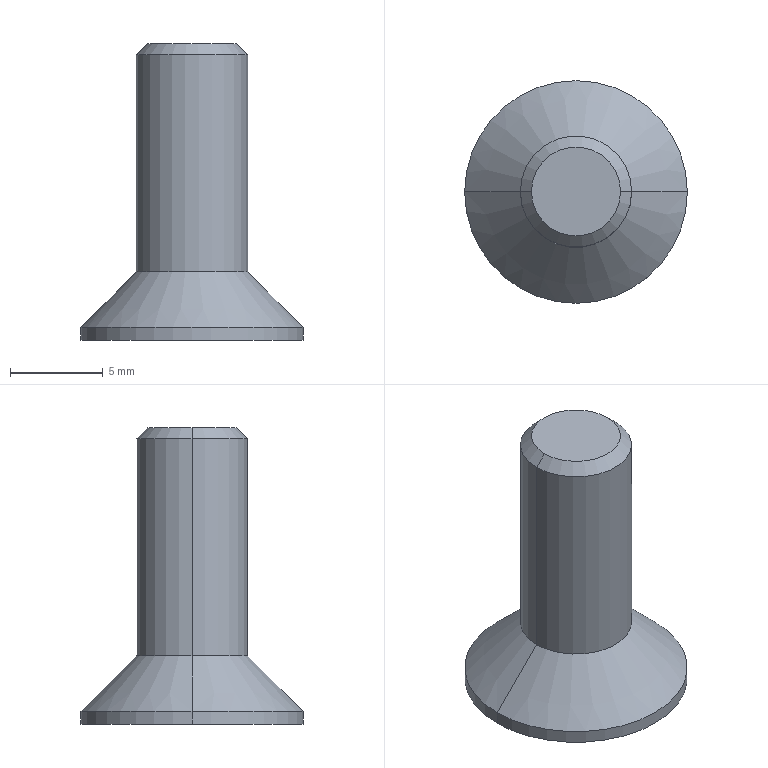Part | STEP file | LE-PJS-M6X16_PN_0003 | 1 solid | 24 faces | box 12 x 12 x 16 mm | volume 571.113 mm3 | plane 14 | cone 6 | cylinder 4 | commonest cylinder face diameters 6 x2 12 x2
STEP:
#1=CARTESIAN_POINT('',(-3.,0.,15.4));
#2=VERTEX_POINT('',#1);
#3=CARTESIAN_POINT('',(3.,0.,15.4));
#4=VERTEX_POINT('',#3);
#5=CARTESIAN_POINT('',(0.,0.,15.4));
#6=DIRECTION('',(0.,0.,-1.));
#7=DIRECTION('',(-1.,0.,0.));
#8=AXIS2_PLACEMENT_3D('',#5,#6,#7);
#9=CIRCLE('',#8,3.);
#10=EDGE_CURVE('',#2,#4,#9,.T.);
#11=ORIENTED_EDGE('',*,*,#10,.T.);
#12=CARTESIAN_POINT('',(3.,0.,3.7));
#13=VERTEX_POINT('',#12);
#14=CARTESIAN_POINT('',(3.,0.,16.));
#15=DIRECTION('',(0.,0.,-1.));
#16=VECTOR('',#15,1000.);
#17=LINE('',#14,#16);
#18=EDGE_CURVE('',#4,#13,#17,.T.);
#19=ORIENTED_EDGE('',*,*,#18,.T.);
#20=CARTESIAN_POINT('',(-3.,0.,3.7));
#21=VERTEX_POINT('',#20);
#22=CARTESIAN_POINT('',(0.,0.,3.7));
#23=DIRECTION('',(0.,0.,1.));
#24=DIRECTION('',(-1.,0.,0.));
#25=AXIS2_PLACEMENT_3D('',#22,#23,#24);
#26=CIRCLE('',#25,3.);
#27=EDGE_CURVE('',#13,#21,#26,.T.);
#28=ORIENTED_EDGE('',*,*,#27,.T.);
#29=CARTESIAN_POINT('',(-3.,0.,16.));
#30=DIRECTION('',(0.,0.,-1.));
#31=VECTOR('',#30,1000.);
#32=LINE('',#29,#31);
#33=EDGE_CURVE('',#2,#21,#32,.T.);
#34=ORIENTED_EDGE('',*,*,#33,.F.);
#35=EDGE_LOOP('',(#11,#19,#28,#34));
#36=FACE_OUTER_BOUND('',#35,.T.);
#37=CARTESIAN_POINT('',(0.,0.,16.));
#38=DIRECTION('',(0.,0.,-1.));
#39=DIRECTION('',(-1.,0.,0.));
#40=AXIS2_PLACEMENT_3D('',#37,#38,#39);
#41=CYLINDRICAL_SURFACE('',#40,3.);
#42=ADVANCED_FACE('',(#36),#41,.T.);
#43=ORIENTED_EDGE('',*,*,#27,.F.);
#44=CARTESIAN_POINT('',(6.,0.,0.7));
#45=VERTEX_POINT('',#44);
#46=CARTESIAN_POINT('',(6.,0.,0.7));
#47=DIRECTION('',(0.7071,0.,-0.7071));
#48=VECTOR('',#47,1000.);
#49=LINE('',#46,#48);
#50=EDGE_CURVE('',#13,#45,#49,.T.);
#51=ORIENTED_EDGE('',*,*,#50,.T.);
#52=CARTESIAN_POINT('',(-6.,0.,0.7));
#53=VERTEX_POINT('',#52);
#54=CARTESIAN_POINT('',(0.,0.,0.7));
#55=DIRECTION('',(0.,0.,1.));
#56=DIRECTION('',(-1.,0.,0.));
#57=AXIS2_PLACEMENT_3D('',#54,#55,#56);
#58=CIRCLE('',#57,6.);
#59=EDGE_CURVE('',#45,#53,#58,.T.);
#60=ORIENTED_EDGE('',*,*,#59,.T.);
#61=CARTESIAN_POINT('',(-6.,0.,0.7));
#62=DIRECTION('',(-0.7071,0.,-0.7071));
#63=VECTOR('',#62,1000.);
#64=LINE('',#61,#63);
#65=EDGE_CURVE('',#21,#53,#64,.T.);
#66=ORIENTED_EDGE('',*,*,#65,.F.);
#67=EDGE_LOOP('',(#43,#51,#60,#66));
#68=FACE_OUTER_BOUND('',#67,.T.);
#69=CARTESIAN_POINT('',(0.,0.,0.7));
#70=DIRECTION('',(0.,0.,-1.));
#71=DIRECTION('',(-1.,0.,0.));
#72=AXIS2_PLACEMENT_3D('',#69,#70,#71);
#73=CONICAL_SURFACE('',#72,6.,0.7854);
#74=ADVANCED_FACE('',(#68),#73,.T.);
#75=CARTESIAN_POINT('',(-2.4,0.,16.));
#76=VERTEX_POINT('',#75);
#77=CARTESIAN_POINT('',(2.4,0.,16.));
#78=VERTEX_POINT('',#77);
#79=CARTESIAN_POINT('',(0.,0.,16.));
#80=DIRECTION('',(0.,0.,-1.));
#81=DIRECTION('',(-1.,0.,0.));
#82=AXIS2_PLACEMENT_3D('',#79,#80,#81);
#83=CIRCLE('',#82,2.4);
#84=EDGE_CURVE('',#76,#78,#83,.T.);
#85=ORIENTED_EDGE('',*,*,#84,.T.);
#86=CARTESIAN_POINT('',(3.,0.,15.4));
#87=DIRECTION('',(0.7071,0.,-0.7071));
#88=VECTOR('',#87,1000.);
#89=LINE('',#86,#88);
#90=EDGE_CURVE('',#78,#4,#89,.T.);
#91=ORIENTED_EDGE('',*,*,#90,.T.);
#92=ORIENTED_EDGE('',*,*,#10,.F.);
#93=CARTESIAN_POINT('',(-3.,0.,15.4));
#94=DIRECTION('',(-0.7071,0.,-0.7071));
#95=VECTOR('',#94,1000.);
#96=LINE('',#93,#95);
#97=EDGE_CURVE('',#76,#2,#96,.T.);
#98=ORIENTED_EDGE('',*,*,#97,.F.);
#99=EDGE_LOOP('',(#85,#91,#92,#98));
#100=FACE_OUTER_BOUND('',#99,.T.);
#101=CARTESIAN_POINT('',(0.,0.,15.4));
#102=DIRECTION('',(0.,0.,-1.));
#103=DIRECTION('',(-1.,0.,0.));
#104=AXIS2_PLACEMENT_3D('',#101,#102,#103);
#105=CONICAL_SURFACE('',#104,3.,0.7854);
#106=ADVANCED_FACE('',(#100),#105,.T.);
#107=ORIENTED_EDGE('',*,*,#59,.F.);
#108=CARTESIAN_POINT('',(6.,0.,0.));
#109=VERTEX_POINT('',#108);
#110=CARTESIAN_POINT('',(6.,0.,3.7));
#111=DIRECTION('',(0.,0.,-1.));
#112=VECTOR('',#111,1000.);
#113=LINE('',#110,#112);
#114=EDGE_CURVE('',#45,#109,#113,.T.);
#115=ORIENTED_EDGE('',*,*,#114,.T.);
#116=CARTESIAN_POINT('',(-6.,0.,0.));
#117=VERTEX_POINT('',#116);
#118=CARTESIAN_POINT('',(0.,0.,0.));
#119=DIRECTION('',(0.,0.,1.));
#120=DIRECTION('',(-1.,0.,0.));
#121=AXIS2_PLACEMENT_3D('',#118,#119,#120);
#122=CIRCLE('',#121,6.);
#123=EDGE_CURVE('',#109,#117,#122,.T.);
#124=ORIENTED_EDGE('',*,*,#123,.T.);
#125=CARTESIAN_POINT('',(-6.,0.,3.7));
#126=DIRECTION('',(0.,0.,-1.));
#127=VECTOR('',#126,1000.);
#128=LINE('',#125,#127);
#129=EDGE_CURVE('',#53,#117,#128,.T.);
#130=ORIENTED_EDGE('',*,*,#129,.F.);
#131=EDGE_LOOP('',(#107,#115,#124,#130));
#132=FACE_OUTER_BOUND('',#131,.T.);
#133=CARTESIAN_POINT('',(0.,0.,3.7));
#134=DIRECTION('',(0.,0.,-1.));
#135=DIRECTION('',(-1.,0.,0.));
#136=AXIS2_PLACEMENT_3D('',#133,#134,#135);
#137=CYLINDRICAL_SURFACE('',#136,6.);
#138=ADVANCED_FACE('',(#132),#137,.T.);
#139=CARTESIAN_POINT('',(0.,0.,3.343));
#140=VERTEX_POINT('',#139);
#141=CARTESIAN_POINT('',(-2.5,0.,1.9));
#142=VERTEX_POINT('',#141);
#143=CARTESIAN_POINT('',(-2.5,0.,1.9));
#144=DIRECTION('',(-0.866,0.,-0.5));
#145=VECTOR('',#144,1000.);
#146=LINE('',#143,#145);
#147=EDGE_CURVE('',#140,#142,#146,.T.);
#148=ORIENTED_EDGE('',*,*,#147,.F.);
#149=CARTESIAN_POINT('',(2.5,0.,1.9));
#150=VERTEX_POINT('',#149);
#151=CARTESIAN_POINT('',(2.5,0.,1.9));
#152=DIRECTION('',(0.866,0.,-0.5));
#153=VECTOR('',#152,1000.);
#154=LINE('',#151,#153);
#155=EDGE_CURVE('',#140,#150,#154,.T.);
#156=ORIENTED_EDGE('',*,*,#155,.T.);
#157=CARTESIAN_POINT('',(2.165,-1.25,1.9));
#158=VERTEX_POINT('',#157);
#159=CARTESIAN_POINT('',(0.,0.,1.9));
#160=DIRECTION('',(0.,0.,1.));
#161=DIRECTION('',(-1.,0.,0.));
#162=AXIS2_PLACEMENT_3D('',#159,#160,#161);
#163=CIRCLE('',#162,2.5);
#164=EDGE_CURVE('',#158,#150,#163,.T.);
#165=ORIENTED_EDGE('',*,*,#164,.F.);
#166=CARTESIAN_POINT('',(0.,-2.5,1.9));
#167=VERTEX_POINT('',#166);
#168=CARTESIAN_POINT('',(0.,0.,1.9));
#169=DIRECTION('',(0.,0.,1.));
#170=DIRECTION('',(-1.,0.,0.));
#171=AXIS2_PLACEMENT_3D('',#168,#169,#170);
#172=CIRCLE('',#171,2.5);
#173=EDGE_CURVE('',#167,#158,#172,.T.);
#174=ORIENTED_EDGE('',*,*,#173,.F.);
#175=CARTESIAN_POINT('',(-2.165,-1.25,1.9));
#176=VERTEX_POINT('',#175);
#177=CARTESIAN_POINT('',(0.,0.,1.9));
#178=DIRECTION('',(0.,0.,1.));
#179=DIRECTION('',(-1.,0.,0.));
#180=AXIS2_PLACEMENT_3D('',#177,#178,#179);
#181=CIRCLE('',#180,2.5);
#182=EDGE_CURVE('',#176,#167,#181,.T.);
#183=ORIENTED_EDGE('',*,*,#182,.F.);
#184=CARTESIAN_POINT('',(0.,0.,1.9));
#185=DIRECTION('',(0.,0.,1.));
#186=DIRECTION('',(-1.,0.,0.));
#187=AXIS2_PLACEMENT_3D('',#184,#185,#186);
#188=CIRCLE('',#187,2.5);
#189=EDGE_CURVE('',#142,#176,#188,.T.);
#190=ORIENTED_EDGE('',*,*,#189,.F.);
#191=EDGE_LOOP('',(#148,#156,#165,#174,#183,#190));
#192=FACE_OUTER_BOUND('',#191,.T.);
#193=CARTESIAN_POINT('',(0.,0.,1.9));
#194=DIRECTION('',(0.,0.,-1.));
#195=DIRECTION('',(-1.,0.,0.));
#196=AXIS2_PLACEMENT_3D('',#193,#194,#195);
#197=CONICAL_SURFACE('',#196,2.5,1.047);
#198=ADVANCED_FACE('',(#192),#197,.F.);
#199=ORIENTED_EDGE('',*,*,#18,.F.);
#200=CARTESIAN_POINT('',(0.,0.,15.4));
#201=DIRECTION('',(0.,0.,-1.));
#202=DIRECTION('',(-1.,0.,0.));
#203=AXIS2_PLACEMENT_3D('',#200,#201,#202);
#204=CIRCLE('',#203,3.);
#205=EDGE_CURVE('',#4,#2,#204,.T.);
#206=ORIENTED_EDGE('',*,*,#205,.T.);
#207=ORIENTED_EDGE('',*,*,#33,.T.);
#208=CARTESIAN_POINT('',(0.,0.,3.7));
#209=DIRECTION('',(0.,0.,1.));
#210=DIRECTION('',(-1.,0.,0.));
#211=AXIS2_PLACEMENT_3D('',#208,#209,#210);
#212=CIRCLE('',#211,3.);
#213=EDGE_CURVE('',#21,#13,#212,.T.);
#214=ORIENTED_EDGE('',*,*,#213,.T.);
#215=EDGE_LOOP('',(#199,#206,#207,#214));
#216=FACE_OUTER_BOUND('',#215,.T.);
#217=CARTESIAN_POINT('',(0.,0.,16.));
#218=DIRECTION('',(0.,0.,-1.));
#219=DIRECTION('',(-1.,0.,0.));
#220=AXIS2_PLACEMENT_3D('',#217,#218,#219);
#221=CYLINDRICAL_SURFACE('',#220,3.);
#222=ADVANCED_FACE('',(#216),#221,.T.);
#223=ORIENTED_EDGE('',*,*,#50,.F.);
#224=ORIENTED_EDGE('',*,*,#213,.F.);
#225=ORIENTED_EDGE('',*,*,#65,.T.);
#226=CARTESIAN_POINT('',(0.,0.,0.7));
#227=DIRECTION('',(0.,0.,1.));
#228=DIRECTION('',(-1.,0.,0.));
#229=AXIS2_PLACEMENT_3D('',#226,#227,#228);
#230=CIRCLE('',#229,6.);
#231=EDGE_CURVE('',#53,#45,#230,.T.);
#232=ORIENTED_EDGE('',*,*,#231,.T.);
#233=EDGE_LOOP('',(#223,#224,#225,#232));
#234=FACE_OUTER_BOUND('',#233,.T.);
#235=CARTESIAN_POINT('',(0.,0.,0.7));
#236=DIRECTION('',(0.,0.,-1.));
#237=DIRECTION('',(-1.,0.,0.));
#238=AXIS2_PLACEMENT_3D('',#235,#236,#237);
#239=CONICAL_SURFACE('',#238,6.,0.7854);
#240=ADVANCED_FACE('',(#234),#239,.T.);
#241=ORIENTED_EDGE('',*,*,#90,.F.);
#242=CARTESIAN_POINT('',(0.,0.,16.));
#243=DIRECTION('',(0.,0.,-1.));
#244=DIRECTION('',(-1.,0.,0.));
#245=AXIS2_PLACEMENT_3D('',#242,#243,#244);
#246=CIRCLE('',#245,2.4);
#247=EDGE_CURVE('',#78,#76,#246,.T.);
#248=ORIENTED_EDGE('',*,*,#247,.T.);
#249=ORIENTED_EDGE('',*,*,#97,.T.);
#250=ORIENTED_EDGE('',*,*,#205,.F.);
#251=EDGE_LOOP('',(#241,#248,#249,#250));
#252=FACE_OUTER_BOUND('',#251,.T.);
#253=CARTESIAN_POINT('',(0.,0.,15.4));
#254=DIRECTION('',(0.,0.,-1.));
#255=DIRECTION('',(-1.,0.,0.));
#256=AXIS2_PLACEMENT_3D('',#253,#254,#255);
#257=CONICAL_SURFACE('',#256,3.,0.7854);
#258=ADVANCED_FACE('',(#252),#257,.T.);
#259=ORIENTED_EDGE('',*,*,#114,.F.);
#260=ORIENTED_EDGE('',*,*,#231,.F.);
#261=ORIENTED_EDGE('',*,*,#129,.T.);
#262=CARTESIAN_POINT('',(0.,0.,0.));
#263=DIRECTION('',(0.,0.,1.));
#264=DIRECTION('',(-1.,0.,0.));
#265=AXIS2_PLACEMENT_3D('',#262,#263,#264);
#266=CIRCLE('',#265,6.);
#267=EDGE_CURVE('',#117,#109,#266,.T.);
#268=ORIENTED_EDGE('',*,*,#267,.T.);
#269=EDGE_LOOP('',(#259,#260,#261,#268));
#270=FACE_OUTER_BOUND('',#269,.T.);
#271=CARTESIAN_POINT('',(0.,0.,3.7));
#272=DIRECTION('',(0.,0.,-1.));
#273=DIRECTION('',(-1.,0.,0.));
#274=AXIS2_PLACEMENT_3D('',#271,#272,#273);
#275=CYLINDRICAL_SURFACE('',#274,6.);
#276=ADVANCED_FACE('',(#270),#275,.T.);
#277=ORIENTED_EDGE('',*,*,#84,.F.);
#278=ORIENTED_EDGE('',*,*,#247,.F.);
#279=EDGE_LOOP('',(#277,#278));
#280=FACE_OUTER_BOUND('',#279,.T.);
#281=CARTESIAN_POINT('',(0.,0.,16.));
#282=DIRECTION('',(0.,0.,1.));
#283=DIRECTION('',(1.,0.,0.));
#284=AXIS2_PLACEMENT_3D('',#281,#282,#283);
#285=PLANE('',#284);
#286=ADVANCED_FACE('',(#280),#285,.T.);
#287=ORIENTED_EDGE('',*,*,#267,.F.);
#288=ORIENTED_EDGE('',*,*,#123,.F.);
#289=EDGE_LOOP('',(#287,#288));
#290=FACE_OUTER_BOUND('',#289,.T.);
#291=CARTESIAN_POINT('',(-2.887,0.,0.));
#292=VERTEX_POINT('',#291);
#293=CARTESIAN_POINT('',(-1.443,2.5,0.));
#294=VERTEX_POINT('',#293);
#295=CARTESIAN_POINT('',(-2.887,0.,0.));
#296=DIRECTION('',(0.5,0.866,0.));
#297=VECTOR('',#296,1000.);
#298=LINE('',#295,#297);
#299=EDGE_CURVE('',#292,#294,#298,.T.);
#300=ORIENTED_EDGE('',*,*,#299,.F.);
#301=CARTESIAN_POINT('',(-1.443,-2.5,0.));
#302=VERTEX_POINT('',#301);
#303=CARTESIAN_POINT('',(-1.443,-2.5,0.));
#304=DIRECTION('',(-0.5,0.866,0.));
#305=VECTOR('',#304,1000.);
#306=LINE('',#303,#305);
#307=EDGE_CURVE('',#302,#292,#306,.T.);
#308=ORIENTED_EDGE('',*,*,#307,.F.);
#309=CARTESIAN_POINT('',(1.443,-2.5,0.));
#310=VERTEX_POINT('',#309);
#311=CARTESIAN_POINT('',(0.,-2.5,0.));
#312=DIRECTION('',(-1.,0.,0.));
#313=VECTOR('',#312,1000.);
#314=LINE('',#311,#313);
#315=EDGE_CURVE('',#310,#302,#314,.T.);
#316=ORIENTED_EDGE('',*,*,#315,.F.);
#317=CARTESIAN_POINT('',(2.887,0.,0.));
#318=VERTEX_POINT('',#317);
#319=CARTESIAN_POINT('',(2.887,0.,0.));
#320=DIRECTION('',(-0.5,-0.866,0.));
#321=VECTOR('',#320,1000.);
#322=LINE('',#319,#321);
#323=EDGE_CURVE('',#318,#310,#322,.T.);
#324=ORIENTED_EDGE('',*,*,#323,.F.);
#325=CARTESIAN_POINT('',(1.443,2.5,0.));
#326=VERTEX_POINT('',#325);
#327=CARTESIAN_POINT('',(1.443,2.5,0.));
#328=DIRECTION('',(0.5,-0.866,0.));
#329=VECTOR('',#328,1000.);
#330=LINE('',#327,#329);
#331=EDGE_CURVE('',#326,#318,#330,.T.);
#332=ORIENTED_EDGE('',*,*,#331,.F.);
#333=CARTESIAN_POINT('',(0.,2.5,0.));
#334=DIRECTION('',(1.,0.,0.));
#335=VECTOR('',#334,1000.);
#336=LINE('',#333,#335);
#337=EDGE_CURVE('',#294,#326,#336,.T.);
#338=ORIENTED_EDGE('',*,*,#337,.F.);
#339=EDGE_LOOP('',(#300,#308,#316,#324,#332,#338));
#340=FACE_BOUND('',#339,.T.);
#341=CARTESIAN_POINT('',(0.,0.,0.));
#342=DIRECTION('',(0.,0.,1.));
#343=DIRECTION('',(1.,0.,0.));
#344=AXIS2_PLACEMENT_3D('',#341,#342,#343);
#345=PLANE('',#344);
#346=ADVANCED_FACE('',(#290,#340),#345,.F.);
#347=CARTESIAN_POINT('',(1.443,2.5,1.9));
#348=VERTEX_POINT('',#347);
#349=CARTESIAN_POINT('',(1.443,2.5,1.9));
#350=DIRECTION('',(0.,0.,-1.));
#351=VECTOR('',#350,1000.);
#352=LINE('',#349,#351);
#353=EDGE_CURVE('',#348,#326,#352,.T.);
#354=ORIENTED_EDGE('',*,*,#353,.F.);
#355=CARTESIAN_POINT('',(0.,2.5,1.9));
#356=VERTEX_POINT('',#355);
#357=CARTESIAN_POINT('',(0.,2.5,1.9));
#358=DIRECTION('',(1.,0.,0.));
#359=VECTOR('',#358,1000.);
#360=LINE('',#357,#359);
#361=EDGE_CURVE('',#356,#348,#360,.T.);
#362=ORIENTED_EDGE('',*,*,#361,.F.);
#363=CARTESIAN_POINT('',(-1.443,2.5,1.9));
#364=VERTEX_POINT('',#363);
#365=CARTESIAN_POINT('',(0.,2.5,1.9));
#366=DIRECTION('',(1.,0.,0.));
#367=VECTOR('',#366,1000.);
#368=LINE('',#365,#367);
#369=EDGE_CURVE('',#364,#356,#368,.T.);
#370=ORIENTED_EDGE('',*,*,#369,.F.);
#371=CARTESIAN_POINT('',(-1.443,2.5,1.9));
#372=DIRECTION('',(0.,0.,1.));
#373=VECTOR('',#372,1000.);
#374=LINE('',#371,#373);
#375=EDGE_CURVE('',#294,#364,#374,.T.);
#376=ORIENTED_EDGE('',*,*,#375,.F.);
#377=ORIENTED_EDGE('',*,*,#337,.T.);
#378=EDGE_LOOP('',(#354,#362,#370,#376,#377));
#379=FACE_OUTER_BOUND('',#378,.T.);
#380=CARTESIAN_POINT('',(-1.443,2.5,1.9));
#381=DIRECTION('',(0.,1.,0.));
#382=DIRECTION('',(0.,0.,1.));
#383=AXIS2_PLACEMENT_3D('',#380,#381,#382);
#384=PLANE('',#383);
#385=ADVANCED_FACE('',(#379),#384,.F.);
#386=ORIENTED_EDGE('',*,*,#375,.T.);
#387=CARTESIAN_POINT('',(-2.165,1.25,1.9));
#388=VERTEX_POINT('',#387);
#389=CARTESIAN_POINT('',(-2.165,1.25,1.9));
#390=DIRECTION('',(0.5,0.866,0.));
#391=VECTOR('',#390,1000.);
#392=LINE('',#389,#391);
#393=EDGE_CURVE('',#388,#364,#392,.T.);
#394=ORIENTED_EDGE('',*,*,#393,.F.);
#395=CARTESIAN_POINT('',(-2.887,0.,1.9));
#396=VERTEX_POINT('',#395);
#397=CARTESIAN_POINT('',(-2.887,0.,1.9));
#398=DIRECTION('',(0.5,0.866,0.));
#399=VECTOR('',#398,1000.);
#400=LINE('',#397,#399);
#401=EDGE_CURVE('',#396,#388,#400,.T.);
#402=ORIENTED_EDGE('',*,*,#401,.F.);
#403=CARTESIAN_POINT('',(-2.887,0.,1.9));
#404=DIRECTION('',(0.,0.,1.));
#405=VECTOR('',#404,1000.);
#406=LINE('',#403,#405);
#407=EDGE_CURVE('',#292,#396,#406,.T.);
#408=ORIENTED_EDGE('',*,*,#407,.F.);
#409=ORIENTED_EDGE('',*,*,#299,.T.);
#410=EDGE_LOOP('',(#386,#394,#402,#408,#409));
#411=FACE_OUTER_BOUND('',#410,.T.);
#412=CARTESIAN_POINT('',(-2.887,0.,1.9));
#413=DIRECTION('',(-0.866,0.5,0.));
#414=DIRECTION('',(-0.5,-0.866,0.));
#415=AXIS2_PLACEMENT_3D('',#412,#413,#414);
#416=PLANE('',#415);
#417=ADVANCED_FACE('',(#411),#416,.F.);
#418=ORIENTED_EDGE('',*,*,#407,.T.);
#419=CARTESIAN_POINT('',(-1.443,-2.5,1.9));
#420=DIRECTION('',(-0.5,0.866,0.));
#421=VECTOR('',#420,1000.);
#422=LINE('',#419,#421);
#423=EDGE_CURVE('',#176,#396,#422,.T.);
#424=ORIENTED_EDGE('',*,*,#423,.F.);
#425=CARTESIAN_POINT('',(-1.443,-2.5,1.9));
#426=VERTEX_POINT('',#425);
#427=CARTESIAN_POINT('',(-1.443,-2.5,1.9));
#428=DIRECTION('',(-0.5,0.866,0.));
#429=VECTOR('',#428,1000.);
#430=LINE('',#427,#429);
#431=EDGE_CURVE('',#426,#176,#430,.T.);
#432=ORIENTED_EDGE('',*,*,#431,.F.);
#433=CARTESIAN_POINT('',(-1.443,-2.5,1.9));
#434=DIRECTION('',(0.,0.,1.));
#435=VECTOR('',#434,1000.);
#436=LINE('',#433,#435);
#437=EDGE_CURVE('',#302,#426,#436,.T.);
#438=ORIENTED_EDGE('',*,*,#437,.F.);
#439=ORIENTED_EDGE('',*,*,#307,.T.);
#440=EDGE_LOOP('',(#418,#424,#432,#438,#439));
#441=FACE_OUTER_BOUND('',#440,.T.);
#442=CARTESIAN_POINT('',(-1.443,-2.5,1.9));
#443=DIRECTION('',(-0.866,-0.5,0.));
#444=DIRECTION('',(0.5,-0.866,0.));
#445=AXIS2_PLACEMENT_3D('',#442,#443,#444);
#446=PLANE('',#445);
#447=ADVANCED_FACE('',(#441),#446,.F.);
#448=ORIENTED_EDGE('',*,*,#437,.T.);
#449=CARTESIAN_POINT('',(0.,-2.5,1.9));
#450=DIRECTION('',(-1.,0.,0.));
#451=VECTOR('',#450,1000.);
#452=LINE('',#449,#451);
#453=EDGE_CURVE('',#167,#426,#452,.T.);
#454=ORIENTED_EDGE('',*,*,#453,.F.);
#455=CARTESIAN_POINT('',(1.443,-2.5,1.9));
#456=VERTEX_POINT('',#455);
#457=CARTESIAN_POINT('',(0.,-2.5,1.9));
#458=DIRECTION('',(-1.,0.,0.));
#459=VECTOR('',#458,1000.);
#460=LINE('',#457,#459);
#461=EDGE_CURVE('',#456,#167,#460,.T.);
#462=ORIENTED_EDGE('',*,*,#461,.F.);
#463=CARTESIAN_POINT('',(1.443,-2.5,1.9));
#464=DIRECTION('',(0.,0.,1.));
#465=VECTOR('',#464,1000.);
#466=LINE('',#463,#465);
#467=EDGE_CURVE('',#310,#456,#466,.T.);
#468=ORIENTED_EDGE('',*,*,#467,.F.);
#469=ORIENTED_EDGE('',*,*,#315,.T.);
#470=EDGE_LOOP('',(#448,#454,#462,#468,#469));
#471=FACE_OUTER_BOUND('',#470,.T.);
#472=CARTESIAN_POINT('',(1.443,-2.5,1.9));
#473=DIRECTION('',(0.,-1.,0.));
#474=DIRECTION('',(1.,0.,0.));
#475=AXIS2_PLACEMENT_3D('',#472,#473,#474);
#476=PLANE('',#475);
#477=ADVANCED_FACE('',(#471),#476,.F.);
#478=ORIENTED_EDGE('',*,*,#467,.T.);
#479=CARTESIAN_POINT('',(2.165,-1.25,1.9));
#480=DIRECTION('',(-0.5,-0.866,0.));
#481=VECTOR('',#480,1000.);
#482=LINE('',#479,#481);
#483=EDGE_CURVE('',#158,#456,#482,.T.);
#484=ORIENTED_EDGE('',*,*,#483,.F.);
#485=CARTESIAN_POINT('',(2.887,0.,1.9));
#486=VERTEX_POINT('',#485);
#487=CARTESIAN_POINT('',(2.887,0.,1.9));
#488=DIRECTION('',(-0.5,-0.866,0.));
#489=VECTOR('',#488,1000.);
#490=LINE('',#487,#489);
#491=EDGE_CURVE('',#486,#158,#490,.T.);
#492=ORIENTED_EDGE('',*,*,#491,.F.);
#493=CARTESIAN_POINT('',(2.887,0.,1.9));
#494=DIRECTION('',(0.,0.,1.));
#495=VECTOR('',#494,1000.);
#496=LINE('',#493,#495);
#497=EDGE_CURVE('',#318,#486,#496,.T.);
#498=ORIENTED_EDGE('',*,*,#497,.F.);
#499=ORIENTED_EDGE('',*,*,#323,.T.);
#500=EDGE_LOOP('',(#478,#484,#492,#498,#499));
#501=FACE_OUTER_BOUND('',#500,.T.);
#502=CARTESIAN_POINT('',(2.887,0.,1.9));
#503=DIRECTION('',(0.866,-0.5,0.));
#504=DIRECTION('',(0.5,0.866,0.));
#505=AXIS2_PLACEMENT_3D('',#502,#503,#504);
#506=PLANE('',#505);
#507=ADVANCED_FACE('',(#501),#506,.F.);
#508=ORIENTED_EDGE('',*,*,#497,.T.);
#509=CARTESIAN_POINT('',(2.165,1.25,1.9));
#510=VERTEX_POINT('',#509);
#511=CARTESIAN_POINT('',(1.443,2.5,1.9));
#512=DIRECTION('',(0.5,-0.866,0.));
#513=VECTOR('',#512,1000.);
#514=LINE('',#511,#513);
#515=EDGE_CURVE('',#510,#486,#514,.T.);
#516=ORIENTED_EDGE('',*,*,#515,.F.);
#517=CARTESIAN_POINT('',(1.443,2.5,1.9));
#518=DIRECTION('',(0.5,-0.866,0.));
#519=VECTOR('',#518,1000.);
#520=LINE('',#517,#519);
#521=EDGE_CURVE('',#348,#510,#520,.T.);
#522=ORIENTED_EDGE('',*,*,#521,.F.);
#523=ORIENTED_EDGE('',*,*,#353,.T.);
#524=ORIENTED_EDGE('',*,*,#331,.T.);
#525=EDGE_LOOP('',(#508,#516,#522,#523,#524));
#526=FACE_OUTER_BOUND('',#525,.T.);
#527=CARTESIAN_POINT('',(1.443,2.5,1.9));
#528=DIRECTION('',(0.866,0.5,0.));
#529=DIRECTION('',(-0.5,0.866,0.));
#530=AXIS2_PLACEMENT_3D('',#527,#528,#529);
#531=PLANE('',#530);
#532=ADVANCED_FACE('',(#526),#531,.F.);
#533=ORIENTED_EDGE('',*,*,#401,.T.);
#534=CARTESIAN_POINT('',(0.,0.,1.9));
#535=DIRECTION('',(0.,0.,1.));
#536=DIRECTION('',(-1.,0.,0.));
#537=AXIS2_PLACEMENT_3D('',#534,#535,#536);
#538=CIRCLE('',#537,2.5);
#539=EDGE_CURVE('',#388,#142,#538,.T.);
#540=ORIENTED_EDGE('',*,*,#539,.T.);
#541=ORIENTED_EDGE('',*,*,#189,.T.);
#542=ORIENTED_EDGE('',*,*,#423,.T.);
#543=EDGE_LOOP('',(#533,#540,#541,#542));
#544=FACE_OUTER_BOUND('',#543,.T.);
#545=CARTESIAN_POINT('',(0.,0.,1.9));
#546=DIRECTION('',(0.,0.,-1.));
#547=DIRECTION('',(-1.,0.,0.));
#548=AXIS2_PLACEMENT_3D('',#545,#546,#547);
#549=PLANE('',#548);
#550=ADVANCED_FACE('',(#544),#549,.T.);
#551=ORIENTED_EDGE('',*,*,#491,.T.);
#552=ORIENTED_EDGE('',*,*,#164,.T.);
#553=CARTESIAN_POINT('',(0.,0.,1.9));
#554=DIRECTION('',(0.,0.,1.));
#555=DIRECTION('',(-1.,0.,0.));
#556=AXIS2_PLACEMENT_3D('',#553,#554,#555);
#557=CIRCLE('',#556,2.5);
#558=EDGE_CURVE('',#150,#510,#557,.T.);
#559=ORIENTED_EDGE('',*,*,#558,.T.);
#560=ORIENTED_EDGE('',*,*,#515,.T.);
#561=EDGE_LOOP('',(#551,#552,#559,#560));
#562=FACE_OUTER_BOUND('',#561,.T.);
#563=CARTESIAN_POINT('',(0.,0.,1.9));
#564=DIRECTION('',(0.,0.,-1.));
#565=DIRECTION('',(-1.,0.,0.));
#566=AXIS2_PLACEMENT_3D('',#563,#564,#565);
#567=PLANE('',#566);
#568=ADVANCED_FACE('',(#562),#567,.T.);
#569=ORIENTED_EDGE('',*,*,#361,.T.);
#570=ORIENTED_EDGE('',*,*,#521,.T.);
#571=CARTESIAN_POINT('',(0.,0.,1.9));
#572=DIRECTION('',(0.,0.,1.));
#573=DIRECTION('',(-1.,0.,0.));
#574=AXIS2_PLACEMENT_3D('',#571,#572,#573);
#575=CIRCLE('',#574,2.5);
#576=EDGE_CURVE('',#510,#356,#575,.T.);
#577=ORIENTED_EDGE('',*,*,#576,.T.);
#578=EDGE_LOOP('',(#569,#570,#577));
#579=FACE_OUTER_BOUND('',#578,.T.);
#580=CARTESIAN_POINT('',(0.,0.,1.9));
#581=DIRECTION('',(0.,0.,-1.));
#582=DIRECTION('',(-1.,0.,0.));
#583=AXIS2_PLACEMENT_3D('',#580,#581,#582);
#584=PLANE('',#583);
#585=ADVANCED_FACE('',(#579),#584,.T.);
#586=ORIENTED_EDGE('',*,*,#155,.F.);
#587=ORIENTED_EDGE('',*,*,#147,.T.);
#588=ORIENTED_EDGE('',*,*,#539,.F.);
#589=CARTESIAN_POINT('',(0.,0.,1.9));
#590=DIRECTION('',(0.,0.,1.));
#591=DIRECTION('',(-1.,0.,0.));
#592=AXIS2_PLACEMENT_3D('',#589,#590,#591);
#593=CIRCLE('',#592,2.5);
#594=EDGE_CURVE('',#356,#388,#593,.T.);
#595=ORIENTED_EDGE('',*,*,#594,.F.);
#596=ORIENTED_EDGE('',*,*,#576,.F.);
#597=ORIENTED_EDGE('',*,*,#558,.F.);
#598=EDGE_LOOP('',(#586,#587,#588,#595,#596,#597));
#599=FACE_OUTER_BOUND('',#598,.T.);
#600=CARTESIAN_POINT('',(0.,0.,1.9));
#601=DIRECTION('',(0.,0.,-1.));
#602=DIRECTION('',(-1.,0.,0.));
#603=AXIS2_PLACEMENT_3D('',#600,#601,#602);
#604=CONICAL_SURFACE('',#603,2.5,1.047);
#605=ADVANCED_FACE('',(#599),#604,.F.);
#606=ORIENTED_EDGE('',*,*,#393,.T.);
#607=ORIENTED_EDGE('',*,*,#369,.T.);
#608=ORIENTED_EDGE('',*,*,#594,.T.);
#609=EDGE_LOOP('',(#606,#607,#608));
#610=FACE_OUTER_BOUND('',#609,.T.);
#611=CARTESIAN_POINT('',(0.,0.,1.9));
#612=DIRECTION('',(0.,0.,-1.));
#613=DIRECTION('',(-1.,0.,0.));
#614=AXIS2_PLACEMENT_3D('',#611,#612,#613);
#615=PLANE('',#614);
#616=ADVANCED_FACE('',(#610),#615,.T.);
#617=ORIENTED_EDGE('',*,*,#483,.T.);
#618=ORIENTED_EDGE('',*,*,#461,.T.);
#619=ORIENTED_EDGE('',*,*,#173,.T.);
#620=EDGE_LOOP('',(#617,#618,#619));
#621=FACE_OUTER_BOUND('',#620,.T.);
#622=CARTESIAN_POINT('',(0.,0.,1.9));
#623=DIRECTION('',(0.,0.,-1.));
#624=DIRECTION('',(-1.,0.,0.));
#625=AXIS2_PLACEMENT_3D('',#622,#623,#624);
#626=PLANE('',#625);
#627=ADVANCED_FACE('',(#621),#626,.T.);
#628=ORIENTED_EDGE('',*,*,#453,.T.);
#629=ORIENTED_EDGE('',*,*,#431,.T.);
#630=ORIENTED_EDGE('',*,*,#182,.T.);
#631=EDGE_LOOP('',(#628,#629,#630));
#632=FACE_OUTER_BOUND('',#631,.T.);
#633=CARTESIAN_POINT('',(0.,0.,1.9));
#634=DIRECTION('',(0.,0.,-1.));
#635=DIRECTION('',(-1.,0.,0.));
#636=AXIS2_PLACEMENT_3D('',#633,#634,#635);
#637=PLANE('',#636);
#638=ADVANCED_FACE('',(#632),#637,.T.);
#639=CLOSED_SHELL('',(#42,#74,#106,#138,#198,#222,#240,#258,#276,#286,#346,#385,#417,#447,#477,#507,#532,#550,#568,#585,#605,#616,#627,#638));
#640=MANIFOLD_SOLID_BREP('',#639);
#641=CARTESIAN_POINT('',(0.,0.,0.));
#642=DIRECTION('',(0.,0.,1.));
#643=DIRECTION('',(1.,0.,0.));
#644=AXIS2_PLACEMENT_3D('',#641,#642,#643);
#645=(LENGTH_UNIT()NAMED_UNIT(*)SI_UNIT(.MILLI.,.METRE.));
#646=UNCERTAINTY_MEASURE_WITH_UNIT(LENGTH_MEASURE(0.00001),#645,'','');
#647=(NAMED_UNIT(*)PLANE_ANGLE_UNIT()SI_UNIT($,.RADIAN.));
#648=(NAMED_UNIT(*)SI_UNIT($,.STERADIAN.)SOLID_ANGLE_UNIT());
#649=(GEOMETRIC_REPRESENTATION_CONTEXT(3)GLOBAL_UNCERTAINTY_ASSIGNED_CONTEXT((#646))GLOBAL_UNIT_ASSIGNED_CONTEXT((#645,#647,#648))REPRESENTATION_CONTEXT('',''));
#650=ADVANCED_BREP_SHAPE_REPRESENTATION('',(#640,#644),#649);